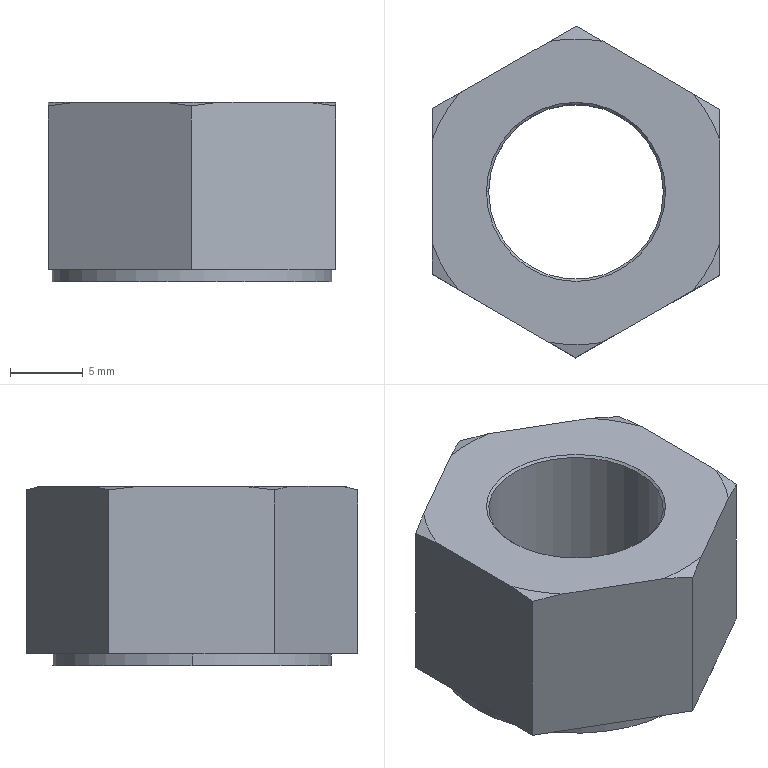Part | STEP file | GB/T1229-1991 high-strength heavy hex nut for steel structures M12 | 1 solid | 23 faces | box 19.773 x 22.78 x 12.3 mm | volume 2715 mm3 | cone 10 | plane 9 | cylinder 4 | commonest cylinder face diameters 12 x2 19.2 x2
STEP:
#1=CARTESIAN_POINT('',(-6.,0.,12.15));
#2=VERTEX_POINT('',#1);
#3=CARTESIAN_POINT('',(6.,0.,12.15));
#4=VERTEX_POINT('',#3);
#5=CARTESIAN_POINT('',(0.,0.,12.15));
#6=DIRECTION('',(0.,0.,1.));
#7=DIRECTION('',(-1.,0.,0.));
#8=AXIS2_PLACEMENT_3D('',#5,#6,#7);
#9=CIRCLE('',#8,6.);
#10=EDGE_CURVE('',#2,#4,#9,.T.);
#11=ORIENTED_EDGE('',*,*,#10,.F.);
#12=CARTESIAN_POINT('',(-6.15,0.,12.3));
#13=VERTEX_POINT('',#12);
#14=CARTESIAN_POINT('',(-6.,0.,12.15));
#15=DIRECTION('',(-0.7071,0.,0.7071));
#16=VECTOR('',#15,1000.);
#17=LINE('',#14,#16);
#18=EDGE_CURVE('',#2,#13,#17,.T.);
#19=ORIENTED_EDGE('',*,*,#18,.T.);
#20=CARTESIAN_POINT('',(6.15,0.,12.3));
#21=VERTEX_POINT('',#20);
#22=CARTESIAN_POINT('',(0.,0.,12.3));
#23=DIRECTION('',(0.,0.,-1.));
#24=DIRECTION('',(-1.,0.,0.));
#25=AXIS2_PLACEMENT_3D('',#22,#23,#24);
#26=CIRCLE('',#25,6.15);
#27=EDGE_CURVE('',#21,#13,#26,.T.);
#28=ORIENTED_EDGE('',*,*,#27,.F.);
#29=CARTESIAN_POINT('',(6.,0.,12.15));
#30=DIRECTION('',(0.7071,0.,0.7071));
#31=VECTOR('',#30,1000.);
#32=LINE('',#29,#31);
#33=EDGE_CURVE('',#4,#21,#32,.T.);
#34=ORIENTED_EDGE('',*,*,#33,.F.);
#35=EDGE_LOOP('',(#11,#19,#28,#34));
#36=FACE_OUTER_BOUND('',#35,.T.);
#37=CARTESIAN_POINT('',(0.,0.,12.15));
#38=DIRECTION('',(0.,0.,1.));
#39=DIRECTION('',(1.,0.,0.));
#40=AXIS2_PLACEMENT_3D('',#37,#38,#39);
#41=CONICAL_SURFACE('',#40,6.,0.7854);
#42=ADVANCED_FACE('',(#36),#41,.F.);
#43=CARTESIAN_POINT('',(6.,0.,0.15));
#44=VERTEX_POINT('',#43);
#45=CARTESIAN_POINT('',(-6.,0.,0.15));
#46=VERTEX_POINT('',#45);
#47=CARTESIAN_POINT('',(0.,0.,0.15));
#48=DIRECTION('',(0.,0.,-1.));
#49=DIRECTION('',(-1.,0.,0.));
#50=AXIS2_PLACEMENT_3D('',#47,#48,#49);
#51=CIRCLE('',#50,6.);
#52=EDGE_CURVE('',#44,#46,#51,.T.);
#53=ORIENTED_EDGE('',*,*,#52,.F.);
#54=CARTESIAN_POINT('',(6.15,0.,0.));
#55=VERTEX_POINT('',#54);
#56=CARTESIAN_POINT('',(6.15,0.,0.));
#57=DIRECTION('',(0.7071,0.,-0.7071));
#58=VECTOR('',#57,1000.);
#59=LINE('',#56,#58);
#60=EDGE_CURVE('',#44,#55,#59,.T.);
#61=ORIENTED_EDGE('',*,*,#60,.T.);
#62=CARTESIAN_POINT('',(-6.15,0.,0.));
#63=VERTEX_POINT('',#62);
#64=CARTESIAN_POINT('',(0.,0.,0.));
#65=DIRECTION('',(0.,0.,1.));
#66=DIRECTION('',(-1.,0.,0.));
#67=AXIS2_PLACEMENT_3D('',#64,#65,#66);
#68=CIRCLE('',#67,6.15);
#69=EDGE_CURVE('',#63,#55,#68,.T.);
#70=ORIENTED_EDGE('',*,*,#69,.F.);
#71=CARTESIAN_POINT('',(-6.15,0.,0.));
#72=DIRECTION('',(-0.7071,0.,-0.7071));
#73=VECTOR('',#72,1000.);
#74=LINE('',#71,#73);
#75=EDGE_CURVE('',#46,#63,#74,.T.);
#76=ORIENTED_EDGE('',*,*,#75,.F.);
#77=EDGE_LOOP('',(#53,#61,#70,#76));
#78=FACE_OUTER_BOUND('',#77,.T.);
#79=CARTESIAN_POINT('',(0.,0.,0.));
#80=DIRECTION('',(0.,0.,-1.));
#81=DIRECTION('',(-1.,0.,0.));
#82=AXIS2_PLACEMENT_3D('',#79,#80,#81);
#83=CONICAL_SURFACE('',#82,6.15,0.7854);
#84=ADVANCED_FACE('',(#78),#83,.F.);
#85=CARTESIAN_POINT('',(-9.6,0.,0.8));
#86=VERTEX_POINT('',#85);
#87=CARTESIAN_POINT('',(9.6,0.,0.8));
#88=VERTEX_POINT('',#87);
#89=CARTESIAN_POINT('',(0.,0.,0.8));
#90=DIRECTION('',(0.,0.,-1.));
#91=DIRECTION('',(-1.,0.,0.));
#92=AXIS2_PLACEMENT_3D('',#89,#90,#91);
#93=CIRCLE('',#92,9.6);
#94=EDGE_CURVE('',#86,#88,#93,.T.);
#95=ORIENTED_EDGE('',*,*,#94,.T.);
#96=CARTESIAN_POINT('',(9.6,0.,0.));
#97=VERTEX_POINT('',#96);
#98=CARTESIAN_POINT('',(9.6,0.,0.8));
#99=DIRECTION('',(0.,0.,-1.));
#100=VECTOR('',#99,1000.);
#101=LINE('',#98,#100);
#102=EDGE_CURVE('',#88,#97,#101,.T.);
#103=ORIENTED_EDGE('',*,*,#102,.T.);
#104=CARTESIAN_POINT('',(-9.6,0.,0.));
#105=VERTEX_POINT('',#104);
#106=CARTESIAN_POINT('',(0.,0.,0.));
#107=DIRECTION('',(0.,0.,-1.));
#108=DIRECTION('',(-1.,0.,0.));
#109=AXIS2_PLACEMENT_3D('',#106,#107,#108);
#110=CIRCLE('',#109,9.6);
#111=EDGE_CURVE('',#105,#97,#110,.T.);
#112=ORIENTED_EDGE('',*,*,#111,.F.);
#113=CARTESIAN_POINT('',(-9.6,0.,0.8));
#114=DIRECTION('',(0.,0.,-1.));
#115=VECTOR('',#114,1000.);
#116=LINE('',#113,#115);
#117=EDGE_CURVE('',#86,#105,#116,.T.);
#118=ORIENTED_EDGE('',*,*,#117,.F.);
#119=EDGE_LOOP('',(#95,#103,#112,#118));
#120=FACE_OUTER_BOUND('',#119,.T.);
#121=CARTESIAN_POINT('',(0.,0.,0.8));
#122=DIRECTION('',(0.,0.,-1.));
#123=DIRECTION('',(-1.,0.,0.));
#124=AXIS2_PLACEMENT_3D('',#121,#122,#123);
#125=CYLINDRICAL_SURFACE('',#124,9.6);
#126=ADVANCED_FACE('',(#120),#125,.T.);
#127=ORIENTED_EDGE('',*,*,#10,.T.);
#128=CARTESIAN_POINT('',(6.,0.,12.3));
#129=DIRECTION('',(0.,0.,-1.));
#130=VECTOR('',#129,1000.);
#131=LINE('',#128,#130);
#132=EDGE_CURVE('',#4,#44,#131,.T.);
#133=ORIENTED_EDGE('',*,*,#132,.T.);
#134=ORIENTED_EDGE('',*,*,#52,.T.);
#135=CARTESIAN_POINT('',(-6.,0.,12.3));
#136=DIRECTION('',(0.,0.,-1.));
#137=VECTOR('',#136,1000.);
#138=LINE('',#135,#137);
#139=EDGE_CURVE('',#2,#46,#138,.T.);
#140=ORIENTED_EDGE('',*,*,#139,.F.);
#141=EDGE_LOOP('',(#127,#133,#134,#140));
#142=FACE_OUTER_BOUND('',#141,.T.);
#143=CARTESIAN_POINT('',(0.,0.,12.3));
#144=DIRECTION('',(0.,0.,-1.));
#145=DIRECTION('',(-1.,0.,0.));
#146=AXIS2_PLACEMENT_3D('',#143,#144,#145);
#147=CYLINDRICAL_SURFACE('',#146,6.);
#148=ADVANCED_FACE('',(#142),#147,.F.);
#149=CARTESIAN_POINT('',(0.0448,11.39,0.8));
#150=VERTEX_POINT('',#149);
#151=CARTESIAN_POINT('',(9.886,5.656,0.8));
#152=VERTEX_POINT('',#151);
#153=CARTESIAN_POINT('',(9.886,5.656,0.8));
#154=DIRECTION('',(0.8641,-0.5034,0.));
#155=VECTOR('',#154,1000.);
#156=LINE('',#153,#155);
#157=EDGE_CURVE('',#150,#152,#156,.T.);
#158=ORIENTED_EDGE('',*,*,#157,.F.);
#159=CARTESIAN_POINT('',(0.0448,11.39,12.062));
#160=VERTEX_POINT('',#159);
#161=CARTESIAN_POINT('',(0.0448,11.39,12.3));
#162=DIRECTION('',(0.,0.,-1.));
#163=VECTOR('',#162,1000.);
#164=LINE('',#161,#163);
#165=EDGE_CURVE('',#160,#150,#164,.T.);
#166=ORIENTED_EDGE('',*,*,#165,.F.);
#167=CARTESIAN_POINT('',(1.856,10.335,12.3));
#168=VERTEX_POINT('',#167);
#169=CARTESIAN_POINT('',(1.856,10.335,12.3));
#170=CARTESIAN_POINT('',(1.25,10.688,12.236));
#171=CARTESIAN_POINT('',(0.6464,11.039,12.155));
#172=CARTESIAN_POINT('',(0.0448,11.39,12.062));
#173=B_SPLINE_CURVE_WITH_KNOTS('',3,(#169,#170,#171,#172),.UNSPECIFIED.,.F.,.F.,(4,4),(0.02083,0.0229),.UNSPECIFIED.);
#174=EDGE_CURVE('',#168,#160,#173,.T.);
#175=ORIENTED_EDGE('',*,*,#174,.F.);
#176=CARTESIAN_POINT('',(8.075,6.711,12.3));
#177=VERTEX_POINT('',#176);
#178=CARTESIAN_POINT('',(9.886,5.656,12.3));
#179=DIRECTION('',(-0.8641,0.5034,0.));
#180=VECTOR('',#179,1000.);
#181=LINE('',#178,#180);
#182=EDGE_CURVE('',#177,#168,#181,.T.);
#183=ORIENTED_EDGE('',*,*,#182,.F.);
#184=CARTESIAN_POINT('',(9.886,5.656,12.062));
#185=VERTEX_POINT('',#184);
#186=CARTESIAN_POINT('',(9.886,5.656,12.062));
#187=CARTESIAN_POINT('',(9.284,6.007,12.155));
#188=CARTESIAN_POINT('',(8.68,6.359,12.236));
#189=CARTESIAN_POINT('',(8.075,6.711,12.3));
#190=B_SPLINE_CURVE_WITH_KNOTS('',3,(#186,#187,#188,#189),.UNSPECIFIED.,.F.,.F.,(4,4),(0.01157,0.01368),.UNSPECIFIED.);
#191=EDGE_CURVE('',#185,#177,#190,.T.);
#192=ORIENTED_EDGE('',*,*,#191,.F.);
#193=CARTESIAN_POINT('',(9.886,5.656,12.3));
#194=DIRECTION('',(0.,0.,-1.));
#195=VECTOR('',#194,1000.);
#196=LINE('',#193,#195);
#197=EDGE_CURVE('',#185,#152,#196,.T.);
#198=ORIENTED_EDGE('',*,*,#197,.T.);
#199=EDGE_LOOP('',(#158,#166,#175,#183,#192,#198));
#200=FACE_OUTER_BOUND('',#199,.T.);
#201=CARTESIAN_POINT('',(9.886,5.656,12.3));
#202=DIRECTION('',(-0.5034,-0.8641,0.));
#203=DIRECTION('',(0.8641,-0.5034,0.));
#204=AXIS2_PLACEMENT_3D('',#201,#202,#203);
#205=PLANE('',#204);
#206=ADVANCED_FACE('',(#200),#205,.F.);
#207=CARTESIAN_POINT('',(-9.842,5.734,0.8));
#208=VERTEX_POINT('',#207);
#209=CARTESIAN_POINT('',(0.0448,11.39,0.8));
#210=DIRECTION('',(0.868,0.4966,0.));
#211=VECTOR('',#210,1000.);
#212=LINE('',#209,#211);
#213=EDGE_CURVE('',#208,#150,#212,.T.);
#214=ORIENTED_EDGE('',*,*,#213,.F.);
#215=CARTESIAN_POINT('',(-9.842,5.734,12.062));
#216=VERTEX_POINT('',#215);
#217=CARTESIAN_POINT('',(-9.842,5.734,12.3));
#218=DIRECTION('',(0.,0.,-1.));
#219=VECTOR('',#218,1000.);
#220=LINE('',#217,#219);
#221=EDGE_CURVE('',#216,#208,#220,.T.);
#222=ORIENTED_EDGE('',*,*,#221,.F.);
#223=CARTESIAN_POINT('',(-8.022,6.775,12.3));
#224=VERTEX_POINT('',#223);
#225=CARTESIAN_POINT('',(-8.022,6.775,12.3));
#226=CARTESIAN_POINT('',(-8.631,6.426,12.236));
#227=CARTESIAN_POINT('',(-9.237,6.08,12.155));
#228=CARTESIAN_POINT('',(-9.842,5.734,12.062));
#229=B_SPLINE_CURVE_WITH_KNOTS('',3,(#225,#226,#227,#228),.UNSPECIFIED.,.F.,.F.,(4,4),(0.02077,0.02285),.UNSPECIFIED.);
#230=EDGE_CURVE('',#224,#216,#229,.T.);
#231=ORIENTED_EDGE('',*,*,#230,.F.);
#232=CARTESIAN_POINT('',(-1.775,10.349,12.3));
#233=VERTEX_POINT('',#232);
#234=CARTESIAN_POINT('',(0.0448,11.39,12.3));
#235=DIRECTION('',(-0.868,-0.4966,0.));
#236=VECTOR('',#235,1000.);
#237=LINE('',#234,#236);
#238=EDGE_CURVE('',#233,#224,#237,.T.);
#239=ORIENTED_EDGE('',*,*,#238,.F.);
#240=CARTESIAN_POINT('',(0.0448,11.39,12.062));
#241=CARTESIAN_POINT('',(-0.5602,11.044,12.155));
#242=CARTESIAN_POINT('',(-1.167,10.697,12.236));
#243=CARTESIAN_POINT('',(-1.775,10.349,12.3));
#244=B_SPLINE_CURVE_WITH_KNOTS('',3,(#240,#241,#242,#243),.UNSPECIFIED.,.F.,.F.,(4,4),(0.01152,0.01363),.UNSPECIFIED.);
#245=EDGE_CURVE('',#160,#233,#244,.T.);
#246=ORIENTED_EDGE('',*,*,#245,.F.);
#247=ORIENTED_EDGE('',*,*,#165,.T.);
#248=EDGE_LOOP('',(#214,#222,#231,#239,#246,#247));
#249=FACE_OUTER_BOUND('',#248,.T.);
#250=CARTESIAN_POINT('',(0.0448,11.39,12.3));
#251=DIRECTION('',(0.4966,-0.868,0.));
#252=DIRECTION('',(0.868,0.4966,0.));
#253=AXIS2_PLACEMENT_3D('',#250,#251,#252);
#254=PLANE('',#253);
#255=ADVANCED_FACE('',(#249),#254,.F.);
#256=CARTESIAN_POINT('',(-9.886,-5.656,0.8));
#257=VERTEX_POINT('',#256);
#258=CARTESIAN_POINT('',(-9.842,5.734,0.8));
#259=DIRECTION('',(0.003934,1.,0.));
#260=VECTOR('',#259,1000.);
#261=LINE('',#258,#260);
#262=EDGE_CURVE('',#257,#208,#261,.T.);
#263=ORIENTED_EDGE('',*,*,#262,.F.);
#264=CARTESIAN_POINT('',(-9.886,-5.656,12.062));
#265=VERTEX_POINT('',#264);
#266=CARTESIAN_POINT('',(-9.886,-5.656,12.3));
#267=DIRECTION('',(0.,0.,-1.));
#268=VECTOR('',#267,1000.);
#269=LINE('',#266,#268);
#270=EDGE_CURVE('',#265,#257,#269,.T.);
#271=ORIENTED_EDGE('',*,*,#270,.F.);
#272=CARTESIAN_POINT('',(-9.878,-3.56,12.3));
#273=VERTEX_POINT('',#272);
#274=CARTESIAN_POINT('',(-9.878,-3.56,12.3));
#275=CARTESIAN_POINT('',(-9.881,-4.261,12.236));
#276=CARTESIAN_POINT('',(-9.884,-4.96,12.155));
#277=CARTESIAN_POINT('',(-9.886,-5.656,12.062));
#278=B_SPLINE_CURVE_WITH_KNOTS('',3,(#274,#275,#276,#277),.UNSPECIFIED.,.F.,.F.,(4,4),(0.01925,0.02132),.UNSPECIFIED.);
#279=EDGE_CURVE('',#273,#265,#278,.T.);
#280=ORIENTED_EDGE('',*,*,#279,.F.);
#281=CARTESIAN_POINT('',(-9.85,3.638,12.3));
#282=VERTEX_POINT('',#281);
#283=CARTESIAN_POINT('',(-9.842,5.734,12.3));
#284=DIRECTION('',(-0.003934,-1.,0.));
#285=VECTOR('',#284,1000.);
#286=LINE('',#283,#285);
#287=EDGE_CURVE('',#282,#273,#286,.T.);
#288=ORIENTED_EDGE('',*,*,#287,.F.);
#289=CARTESIAN_POINT('',(-9.842,5.734,12.062));
#290=CARTESIAN_POINT('',(-9.844,5.037,12.155));
#291=CARTESIAN_POINT('',(-9.847,4.338,12.236));
#292=CARTESIAN_POINT('',(-9.85,3.638,12.3));
#293=B_SPLINE_CURVE_WITH_KNOTS('',3,(#289,#290,#291,#292),.UNSPECIFIED.,.F.,.F.,(4,4),(0.009986,0.0121),.UNSPECIFIED.);
#294=EDGE_CURVE('',#216,#282,#293,.T.);
#295=ORIENTED_EDGE('',*,*,#294,.F.);
#296=ORIENTED_EDGE('',*,*,#221,.T.);
#297=EDGE_LOOP('',(#263,#271,#280,#288,#295,#296));
#298=FACE_OUTER_BOUND('',#297,.T.);
#299=CARTESIAN_POINT('',(-9.842,5.734,12.3));
#300=DIRECTION('',(1.,-0.003934,0.));
#301=DIRECTION('',(0.003934,1.,0.));
#302=AXIS2_PLACEMENT_3D('',#299,#300,#301);
#303=PLANE('',#302);
#304=ADVANCED_FACE('',(#298),#303,.F.);
#305=CARTESIAN_POINT('',(-0.0448,-11.39,0.8));
#306=VERTEX_POINT('',#305);
#307=CARTESIAN_POINT('',(-9.886,-5.656,0.8));
#308=DIRECTION('',(-0.8641,0.5034,0.));
#309=VECTOR('',#308,1000.);
#310=LINE('',#307,#309);
#311=EDGE_CURVE('',#306,#257,#310,.T.);
#312=ORIENTED_EDGE('',*,*,#311,.F.);
#313=CARTESIAN_POINT('',(-0.0448,-11.39,12.062));
#314=VERTEX_POINT('',#313);
#315=CARTESIAN_POINT('',(-0.0448,-11.39,12.3));
#316=DIRECTION('',(0.,0.,-1.));
#317=VECTOR('',#316,1000.);
#318=LINE('',#315,#317);
#319=EDGE_CURVE('',#314,#306,#318,.T.);
#320=ORIENTED_EDGE('',*,*,#319,.F.);
#321=CARTESIAN_POINT('',(-1.856,-10.335,12.3));
#322=VERTEX_POINT('',#321);
#323=CARTESIAN_POINT('',(-1.856,-10.335,12.3));
#324=CARTESIAN_POINT('',(-1.25,-10.688,12.236));
#325=CARTESIAN_POINT('',(-0.6464,-11.039,12.155));
#326=CARTESIAN_POINT('',(-0.0448,-11.39,12.062));
#327=B_SPLINE_CURVE_WITH_KNOTS('',3,(#323,#324,#325,#326),.UNSPECIFIED.,.F.,.F.,(4,4),(0.02083,0.0229),.UNSPECIFIED.);
#328=EDGE_CURVE('',#322,#314,#327,.T.);
#329=ORIENTED_EDGE('',*,*,#328,.F.);
#330=CARTESIAN_POINT('',(-8.075,-6.711,12.3));
#331=VERTEX_POINT('',#330);
#332=CARTESIAN_POINT('',(-9.886,-5.656,12.3));
#333=DIRECTION('',(0.8641,-0.5034,0.));
#334=VECTOR('',#333,1000.);
#335=LINE('',#332,#334);
#336=EDGE_CURVE('',#331,#322,#335,.T.);
#337=ORIENTED_EDGE('',*,*,#336,.F.);
#338=CARTESIAN_POINT('',(-9.886,-5.656,12.062));
#339=CARTESIAN_POINT('',(-9.284,-6.007,12.155));
#340=CARTESIAN_POINT('',(-8.68,-6.359,12.236));
#341=CARTESIAN_POINT('',(-8.075,-6.711,12.3));
#342=B_SPLINE_CURVE_WITH_KNOTS('',3,(#338,#339,#340,#341),.UNSPECIFIED.,.F.,.F.,(4,4),(0.01157,0.01368),.UNSPECIFIED.);
#343=EDGE_CURVE('',#265,#331,#342,.T.);
#344=ORIENTED_EDGE('',*,*,#343,.F.);
#345=ORIENTED_EDGE('',*,*,#270,.T.);
#346=EDGE_LOOP('',(#312,#320,#329,#337,#344,#345));
#347=FACE_OUTER_BOUND('',#346,.T.);
#348=CARTESIAN_POINT('',(-9.886,-5.656,12.3));
#349=DIRECTION('',(0.5034,0.8641,0.));
#350=DIRECTION('',(-0.8641,0.5034,0.));
#351=AXIS2_PLACEMENT_3D('',#348,#349,#350);
#352=PLANE('',#351);
#353=ADVANCED_FACE('',(#347),#352,.F.);
#354=CARTESIAN_POINT('',(9.842,-5.734,0.8));
#355=VERTEX_POINT('',#354);
#356=CARTESIAN_POINT('',(-0.0448,-11.39,0.8));
#357=DIRECTION('',(-0.868,-0.4966,0.));
#358=VECTOR('',#357,1000.);
#359=LINE('',#356,#358);
#360=EDGE_CURVE('',#355,#306,#359,.T.);
#361=ORIENTED_EDGE('',*,*,#360,.F.);
#362=CARTESIAN_POINT('',(9.842,-5.734,12.062));
#363=VERTEX_POINT('',#362);
#364=CARTESIAN_POINT('',(9.842,-5.734,12.3));
#365=DIRECTION('',(0.,0.,-1.));
#366=VECTOR('',#365,1000.);
#367=LINE('',#364,#366);
#368=EDGE_CURVE('',#363,#355,#367,.T.);
#369=ORIENTED_EDGE('',*,*,#368,.F.);
#370=CARTESIAN_POINT('',(8.022,-6.775,12.3));
#371=VERTEX_POINT('',#370);
#372=CARTESIAN_POINT('',(8.022,-6.775,12.3));
#373=CARTESIAN_POINT('',(8.631,-6.426,12.236));
#374=CARTESIAN_POINT('',(9.237,-6.08,12.155));
#375=CARTESIAN_POINT('',(9.842,-5.734,12.062));
#376=B_SPLINE_CURVE_WITH_KNOTS('',3,(#372,#373,#374,#375),.UNSPECIFIED.,.F.,.F.,(4,4),(0.02077,0.02285),.UNSPECIFIED.);
#377=EDGE_CURVE('',#371,#363,#376,.T.);
#378=ORIENTED_EDGE('',*,*,#377,.F.);
#379=CARTESIAN_POINT('',(1.775,-10.349,12.3));
#380=VERTEX_POINT('',#379);
#381=CARTESIAN_POINT('',(-0.0448,-11.39,12.3));
#382=DIRECTION('',(0.868,0.4966,0.));
#383=VECTOR('',#382,1000.);
#384=LINE('',#381,#383);
#385=EDGE_CURVE('',#380,#371,#384,.T.);
#386=ORIENTED_EDGE('',*,*,#385,.F.);
#387=CARTESIAN_POINT('',(-0.0448,-11.39,12.062));
#388=CARTESIAN_POINT('',(0.5602,-11.044,12.155));
#389=CARTESIAN_POINT('',(1.167,-10.697,12.236));
#390=CARTESIAN_POINT('',(1.775,-10.349,12.3));
#391=B_SPLINE_CURVE_WITH_KNOTS('',3,(#387,#388,#389,#390),.UNSPECIFIED.,.F.,.F.,(4,4),(0.01152,0.01363),.UNSPECIFIED.);
#392=EDGE_CURVE('',#314,#380,#391,.T.);
#393=ORIENTED_EDGE('',*,*,#392,.F.);
#394=ORIENTED_EDGE('',*,*,#319,.T.);
#395=EDGE_LOOP('',(#361,#369,#378,#386,#393,#394));
#396=FACE_OUTER_BOUND('',#395,.T.);
#397=CARTESIAN_POINT('',(-0.0448,-11.39,12.3));
#398=DIRECTION('',(-0.4966,0.868,0.));
#399=DIRECTION('',(-0.868,-0.4966,0.));
#400=AXIS2_PLACEMENT_3D('',#397,#398,#399);
#401=PLANE('',#400);
#402=ADVANCED_FACE('',(#396),#401,.F.);
#403=CARTESIAN_POINT('',(9.842,-5.734,0.8));
#404=DIRECTION('',(-0.003934,-1.,0.));
#405=VECTOR('',#404,1000.);
#406=LINE('',#403,#405);
#407=EDGE_CURVE('',#152,#355,#406,.T.);
#408=ORIENTED_EDGE('',*,*,#407,.F.);
#409=ORIENTED_EDGE('',*,*,#197,.F.);
#410=CARTESIAN_POINT('',(9.878,3.56,12.3));
#411=VERTEX_POINT('',#410);
#412=CARTESIAN_POINT('',(9.878,3.56,12.3));
#413=CARTESIAN_POINT('',(9.881,4.261,12.236));
#414=CARTESIAN_POINT('',(9.884,4.96,12.155));
#415=CARTESIAN_POINT('',(9.886,5.656,12.062));
#416=B_SPLINE_CURVE_WITH_KNOTS('',3,(#412,#413,#414,#415),.UNSPECIFIED.,.F.,.F.,(4,4),(0.01925,0.02132),.UNSPECIFIED.);
#417=EDGE_CURVE('',#411,#185,#416,.T.);
#418=ORIENTED_EDGE('',*,*,#417,.F.);
#419=CARTESIAN_POINT('',(9.85,-3.638,12.3));
#420=VERTEX_POINT('',#419);
#421=CARTESIAN_POINT('',(9.842,-5.734,12.3));
#422=DIRECTION('',(0.003934,1.,0.));
#423=VECTOR('',#422,1000.);
#424=LINE('',#421,#423);
#425=EDGE_CURVE('',#420,#411,#424,.T.);
#426=ORIENTED_EDGE('',*,*,#425,.F.);
#427=CARTESIAN_POINT('',(9.842,-5.734,12.062));
#428=CARTESIAN_POINT('',(9.844,-5.037,12.155));
#429=CARTESIAN_POINT('',(9.847,-4.338,12.236));
#430=CARTESIAN_POINT('',(9.85,-3.638,12.3));
#431=B_SPLINE_CURVE_WITH_KNOTS('',3,(#427,#428,#429,#430),.UNSPECIFIED.,.F.,.F.,(4,4),(0.009986,0.0121),.UNSPECIFIED.);
#432=EDGE_CURVE('',#363,#420,#431,.T.);
#433=ORIENTED_EDGE('',*,*,#432,.F.);
#434=ORIENTED_EDGE('',*,*,#368,.T.);
#435=EDGE_LOOP('',(#408,#409,#418,#426,#433,#434));
#436=FACE_OUTER_BOUND('',#435,.T.);
#437=CARTESIAN_POINT('',(9.842,-5.734,12.3));
#438=DIRECTION('',(-1.,0.003934,0.));
#439=DIRECTION('',(-0.003934,-1.,0.));
#440=AXIS2_PLACEMENT_3D('',#437,#438,#439);
#441=PLANE('',#440);
#442=ADVANCED_FACE('',(#436),#441,.F.);
#443=ORIENTED_EDGE('',*,*,#69,.T.);
#444=CARTESIAN_POINT('',(0.,0.,0.));
#445=DIRECTION('',(0.,0.,1.));
#446=DIRECTION('',(-1.,0.,0.));
#447=AXIS2_PLACEMENT_3D('',#444,#445,#446);
#448=CIRCLE('',#447,6.15);
#449=EDGE_CURVE('',#55,#63,#448,.T.);
#450=ORIENTED_EDGE('',*,*,#449,.T.);
#451=EDGE_LOOP('',(#443,#450));
#452=FACE_BOUND('',#451,.T.);
#453=ORIENTED_EDGE('',*,*,#111,.T.);
#454=CARTESIAN_POINT('',(0.,0.,0.));
#455=DIRECTION('',(0.,0.,-1.));
#456=DIRECTION('',(-1.,0.,0.));
#457=AXIS2_PLACEMENT_3D('',#454,#455,#456);
#458=CIRCLE('',#457,9.6);
#459=EDGE_CURVE('',#97,#105,#458,.T.);
#460=ORIENTED_EDGE('',*,*,#459,.T.);
#461=EDGE_LOOP('',(#453,#460));
#462=FACE_OUTER_BOUND('',#461,.T.);
#463=CARTESIAN_POINT('',(9.886,5.656,0.));
#464=DIRECTION('',(0.,0.,-1.));
#465=DIRECTION('',(-1.,0.,0.));
#466=AXIS2_PLACEMENT_3D('',#463,#464,#465);
#467=PLANE('',#466);
#468=ADVANCED_FACE('',(#452,#462),#467,.T.);
#469=ORIENTED_EDGE('',*,*,#27,.T.);
#470=CARTESIAN_POINT('',(0.,0.,12.3));
#471=DIRECTION('',(0.,0.,-1.));
#472=DIRECTION('',(-1.,0.,0.));
#473=AXIS2_PLACEMENT_3D('',#470,#471,#472);
#474=CIRCLE('',#473,6.15);
#475=EDGE_CURVE('',#13,#21,#474,.T.);
#476=ORIENTED_EDGE('',*,*,#475,.T.);
#477=EDGE_LOOP('',(#469,#476));
#478=FACE_BOUND('',#477,.T.);
#479=CARTESIAN_POINT('',(0.,0.,12.3));
#480=DIRECTION('',(0.,0.,1.));
#481=DIRECTION('',(1.,0.,0.));
#482=AXIS2_PLACEMENT_3D('',#479,#480,#481);
#483=CIRCLE('',#482,10.5);
#484=EDGE_CURVE('',#224,#282,#483,.T.);
#485=ORIENTED_EDGE('',*,*,#484,.T.);
#486=ORIENTED_EDGE('',*,*,#287,.T.);
#487=CARTESIAN_POINT('',(0.,0.,12.3));
#488=DIRECTION('',(0.,0.,1.));
#489=DIRECTION('',(1.,0.,0.));
#490=AXIS2_PLACEMENT_3D('',#487,#488,#489);
#491=CIRCLE('',#490,10.5);
#492=EDGE_CURVE('',#273,#331,#491,.T.);
#493=ORIENTED_EDGE('',*,*,#492,.T.);
#494=ORIENTED_EDGE('',*,*,#336,.T.);
#495=CARTESIAN_POINT('',(0.,0.,12.3));
#496=DIRECTION('',(0.,0.,1.));
#497=DIRECTION('',(1.,0.,0.));
#498=AXIS2_PLACEMENT_3D('',#495,#496,#497);
#499=CIRCLE('',#498,10.5);
#500=EDGE_CURVE('',#322,#380,#499,.T.);
#501=ORIENTED_EDGE('',*,*,#500,.T.);
#502=ORIENTED_EDGE('',*,*,#385,.T.);
#503=CARTESIAN_POINT('',(0.,0.,12.3));
#504=DIRECTION('',(0.,0.,1.));
#505=DIRECTION('',(1.,0.,0.));
#506=AXIS2_PLACEMENT_3D('',#503,#504,#505);
#507=CIRCLE('',#506,10.5);
#508=EDGE_CURVE('',#371,#420,#507,.T.);
#509=ORIENTED_EDGE('',*,*,#508,.T.);
#510=ORIENTED_EDGE('',*,*,#425,.T.);
#511=CARTESIAN_POINT('',(0.,0.,12.3));
#512=DIRECTION('',(0.,0.,1.));
#513=DIRECTION('',(1.,0.,0.));
#514=AXIS2_PLACEMENT_3D('',#511,#512,#513);
#515=CIRCLE('',#514,10.5);
#516=EDGE_CURVE('',#411,#177,#515,.T.);
#517=ORIENTED_EDGE('',*,*,#516,.T.);
#518=ORIENTED_EDGE('',*,*,#182,.T.);
#519=CARTESIAN_POINT('',(0.,0.,12.3));
#520=DIRECTION('',(0.,0.,1.));
#521=DIRECTION('',(1.,0.,0.));
#522=AXIS2_PLACEMENT_3D('',#519,#520,#521);
#523=CIRCLE('',#522,10.5);
#524=EDGE_CURVE('',#168,#233,#523,.T.);
#525=ORIENTED_EDGE('',*,*,#524,.T.);
#526=ORIENTED_EDGE('',*,*,#238,.T.);
#527=EDGE_LOOP('',(#485,#486,#493,#494,#501,#502,#509,#510,#517,#518,#525,#526));
#528=FACE_OUTER_BOUND('',#527,.T.);
#529=CARTESIAN_POINT('',(9.886,5.656,12.3));
#530=DIRECTION('',(0.,0.,-1.));
#531=DIRECTION('',(-1.,0.,0.));
#532=AXIS2_PLACEMENT_3D('',#529,#530,#531);
#533=PLANE('',#532);
#534=ADVANCED_FACE('',(#478,#528),#533,.F.);
#535=ORIENTED_EDGE('',*,*,#132,.F.);
#536=CARTESIAN_POINT('',(0.,0.,12.15));
#537=DIRECTION('',(0.,0.,1.));
#538=DIRECTION('',(-1.,0.,0.));
#539=AXIS2_PLACEMENT_3D('',#536,#537,#538);
#540=CIRCLE('',#539,6.);
#541=EDGE_CURVE('',#4,#2,#540,.T.);
#542=ORIENTED_EDGE('',*,*,#541,.T.);
#543=ORIENTED_EDGE('',*,*,#139,.T.);
#544=CARTESIAN_POINT('',(0.,0.,0.15));
#545=DIRECTION('',(0.,0.,-1.));
#546=DIRECTION('',(-1.,0.,0.));
#547=AXIS2_PLACEMENT_3D('',#544,#545,#546);
#548=CIRCLE('',#547,6.);
#549=EDGE_CURVE('',#46,#44,#548,.T.);
#550=ORIENTED_EDGE('',*,*,#549,.T.);
#551=EDGE_LOOP('',(#535,#542,#543,#550));
#552=FACE_OUTER_BOUND('',#551,.T.);
#553=CARTESIAN_POINT('',(0.,0.,12.3));
#554=DIRECTION('',(0.,0.,-1.));
#555=DIRECTION('',(-1.,0.,0.));
#556=AXIS2_PLACEMENT_3D('',#553,#554,#555);
#557=CYLINDRICAL_SURFACE('',#556,6.);
#558=ADVANCED_FACE('',(#552),#557,.F.);
#559=ORIENTED_EDGE('',*,*,#191,.T.);
#560=ORIENTED_EDGE('',*,*,#516,.F.);
#561=ORIENTED_EDGE('',*,*,#417,.T.);
#562=EDGE_LOOP('',(#559,#560,#561));
#563=FACE_OUTER_BOUND('',#562,.T.);
#564=CARTESIAN_POINT('',(0.,0.,12.3));
#565=DIRECTION('',(0.,0.,-1.));
#566=DIRECTION('',(1.,0.,0.));
#567=AXIS2_PLACEMENT_3D('',#564,#565,#566);
#568=CONICAL_SURFACE('',#567,10.5,1.309);
#569=ADVANCED_FACE('',(#563),#568,.T.);
#570=ORIENTED_EDGE('',*,*,#377,.T.);
#571=ORIENTED_EDGE('',*,*,#432,.T.);
#572=ORIENTED_EDGE('',*,*,#508,.F.);
#573=EDGE_LOOP('',(#570,#571,#572));
#574=FACE_OUTER_BOUND('',#573,.T.);
#575=CARTESIAN_POINT('',(0.,0.,12.3));
#576=DIRECTION('',(0.,0.,-1.));
#577=DIRECTION('',(1.,0.,0.));
#578=AXIS2_PLACEMENT_3D('',#575,#576,#577);
#579=CONICAL_SURFACE('',#578,10.5,1.309);
#580=ADVANCED_FACE('',(#574),#579,.T.);
#581=ORIENTED_EDGE('',*,*,#328,.T.);
#582=ORIENTED_EDGE('',*,*,#392,.T.);
#583=ORIENTED_EDGE('',*,*,#500,.F.);
#584=EDGE_LOOP('',(#581,#582,#583));
#585=FACE_OUTER_BOUND('',#584,.T.);
#586=CARTESIAN_POINT('',(0.,0.,12.3));
#587=DIRECTION('',(0.,0.,-1.));
#588=DIRECTION('',(1.,0.,0.));
#589=AXIS2_PLACEMENT_3D('',#586,#587,#588);
#590=CONICAL_SURFACE('',#589,10.5,1.309);
#591=ADVANCED_FACE('',(#585),#590,.T.);
#592=ORIENTED_EDGE('',*,*,#279,.T.);
#593=ORIENTED_EDGE('',*,*,#343,.T.);
#594=ORIENTED_EDGE('',*,*,#492,.F.);
#595=EDGE_LOOP('',(#592,#593,#594));
#596=FACE_OUTER_BOUND('',#595,.T.);
#597=CARTESIAN_POINT('',(0.,0.,12.3));
#598=DIRECTION('',(0.,0.,-1.));
#599=DIRECTION('',(1.,0.,0.));
#600=AXIS2_PLACEMENT_3D('',#597,#598,#599);
#601=CONICAL_SURFACE('',#600,10.5,1.309);
#602=ADVANCED_FACE('',(#596),#601,.T.);
#603=ORIENTED_EDGE('',*,*,#230,.T.);
#604=ORIENTED_EDGE('',*,*,#294,.T.);
#605=ORIENTED_EDGE('',*,*,#484,.F.);
#606=EDGE_LOOP('',(#603,#604,#605));
#607=FACE_OUTER_BOUND('',#606,.T.);
#608=CARTESIAN_POINT('',(0.,0.,12.3));
#609=DIRECTION('',(0.,0.,-1.));
#610=DIRECTION('',(1.,0.,0.));
#611=AXIS2_PLACEMENT_3D('',#608,#609,#610);
#612=CONICAL_SURFACE('',#611,10.5,1.309);
#613=ADVANCED_FACE('',(#607),#612,.T.);
#614=ORIENTED_EDGE('',*,*,#174,.T.);
#615=ORIENTED_EDGE('',*,*,#245,.T.);
#616=ORIENTED_EDGE('',*,*,#524,.F.);
#617=EDGE_LOOP('',(#614,#615,#616));
#618=FACE_OUTER_BOUND('',#617,.T.);
#619=CARTESIAN_POINT('',(0.,0.,12.3));
#620=DIRECTION('',(0.,0.,-1.));
#621=DIRECTION('',(1.,0.,0.));
#622=AXIS2_PLACEMENT_3D('',#619,#620,#621);
#623=CONICAL_SURFACE('',#622,10.5,1.309);
#624=ADVANCED_FACE('',(#618),#623,.T.);
#625=ORIENTED_EDGE('',*,*,#94,.F.);
#626=CARTESIAN_POINT('',(0.,0.,0.8));
#627=DIRECTION('',(0.,0.,-1.));
#628=DIRECTION('',(-1.,0.,0.));
#629=AXIS2_PLACEMENT_3D('',#626,#627,#628);
#630=CIRCLE('',#629,9.6);
#631=EDGE_CURVE('',#88,#86,#630,.T.);
#632=ORIENTED_EDGE('',*,*,#631,.F.);
#633=EDGE_LOOP('',(#625,#632));
#634=FACE_BOUND('',#633,.T.);
#635=ORIENTED_EDGE('',*,*,#157,.T.);
#636=ORIENTED_EDGE('',*,*,#407,.T.);
#637=ORIENTED_EDGE('',*,*,#360,.T.);
#638=ORIENTED_EDGE('',*,*,#311,.T.);
#639=ORIENTED_EDGE('',*,*,#262,.T.);
#640=ORIENTED_EDGE('',*,*,#213,.T.);
#641=EDGE_LOOP('',(#635,#636,#637,#638,#639,#640));
#642=FACE_OUTER_BOUND('',#641,.T.);
#643=CARTESIAN_POINT('',(0.,0.,0.8));
#644=DIRECTION('',(0.,0.,-1.));
#645=DIRECTION('',(-1.,0.,0.));
#646=AXIS2_PLACEMENT_3D('',#643,#644,#645);
#647=PLANE('',#646);
#648=ADVANCED_FACE('',(#634,#642),#647,.T.);
#649=ORIENTED_EDGE('',*,*,#102,.F.);
#650=ORIENTED_EDGE('',*,*,#631,.T.);
#651=ORIENTED_EDGE('',*,*,#117,.T.);
#652=ORIENTED_EDGE('',*,*,#459,.F.);
#653=EDGE_LOOP('',(#649,#650,#651,#652));
#654=FACE_OUTER_BOUND('',#653,.T.);
#655=CARTESIAN_POINT('',(0.,0.,0.8));
#656=DIRECTION('',(0.,0.,-1.));
#657=DIRECTION('',(-1.,0.,0.));
#658=AXIS2_PLACEMENT_3D('',#655,#656,#657);
#659=CYLINDRICAL_SURFACE('',#658,9.6);
#660=ADVANCED_FACE('',(#654),#659,.T.);
#661=ORIENTED_EDGE('',*,*,#60,.F.);
#662=ORIENTED_EDGE('',*,*,#549,.F.);
#663=ORIENTED_EDGE('',*,*,#75,.T.);
#664=ORIENTED_EDGE('',*,*,#449,.F.);
#665=EDGE_LOOP('',(#661,#662,#663,#664));
#666=FACE_OUTER_BOUND('',#665,.T.);
#667=CARTESIAN_POINT('',(0.,0.,0.));
#668=DIRECTION('',(0.,0.,-1.));
#669=DIRECTION('',(-1.,0.,0.));
#670=AXIS2_PLACEMENT_3D('',#667,#668,#669);
#671=CONICAL_SURFACE('',#670,6.15,0.7854);
#672=ADVANCED_FACE('',(#666),#671,.F.);
#673=ORIENTED_EDGE('',*,*,#18,.F.);
#674=ORIENTED_EDGE('',*,*,#541,.F.);
#675=ORIENTED_EDGE('',*,*,#33,.T.);
#676=ORIENTED_EDGE('',*,*,#475,.F.);
#677=EDGE_LOOP('',(#673,#674,#675,#676));
#678=FACE_OUTER_BOUND('',#677,.T.);
#679=CARTESIAN_POINT('',(0.,0.,12.15));
#680=DIRECTION('',(0.,0.,1.));
#681=DIRECTION('',(1.,0.,0.));
#682=AXIS2_PLACEMENT_3D('',#679,#680,#681);
#683=CONICAL_SURFACE('',#682,6.,0.7854);
#684=ADVANCED_FACE('',(#678),#683,.F.);
#685=CLOSED_SHELL('',(#42,#84,#126,#148,#206,#255,#304,#353,#402,#442,#468,#534,#558,#569,#580,#591,#602,#613,#624,#648,#660,#672,#684));
#686=MANIFOLD_SOLID_BREP('',#685);
#687=CARTESIAN_POINT('',(0.,0.,0.));
#688=DIRECTION('',(0.,0.,1.));
#689=DIRECTION('',(1.,0.,0.));
#690=AXIS2_PLACEMENT_3D('',#687,#688,#689);
#691=(LENGTH_UNIT()NAMED_UNIT(*)SI_UNIT(.MILLI.,.METRE.));
#692=UNCERTAINTY_MEASURE_WITH_UNIT(LENGTH_MEASURE(0.00001),#691,'','');
#693=(NAMED_UNIT(*)PLANE_ANGLE_UNIT()SI_UNIT($,.RADIAN.));
#694=(NAMED_UNIT(*)SI_UNIT($,.STERADIAN.)SOLID_ANGLE_UNIT());
#695=(GEOMETRIC_REPRESENTATION_CONTEXT(3)GLOBAL_UNCERTAINTY_ASSIGNED_CONTEXT((#692))GLOBAL_UNIT_ASSIGNED_CONTEXT((#691,#693,#694))REPRESENTATION_CONTEXT('',''));
#696=ADVANCED_BREP_SHAPE_REPRESENTATION('',(#686,#690),#695);